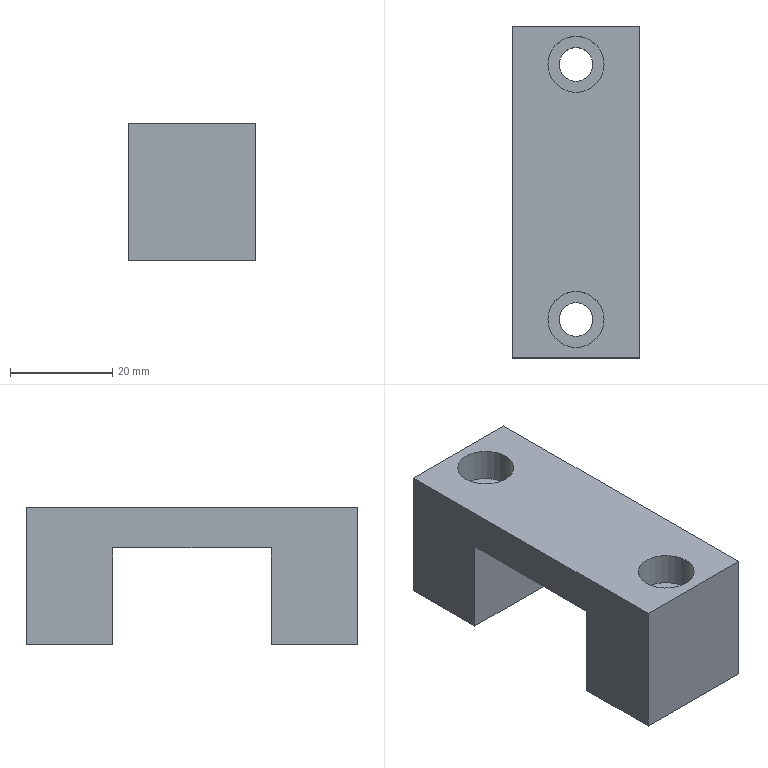Part | STEP file | solid 238 | 1 solid | 16 faces | box 25 x 65 x 27 mm | volume 26512 mm3 | plane 12 | cylinder 4 | commonest cylinder face diameters 6.6 x2 11 x2